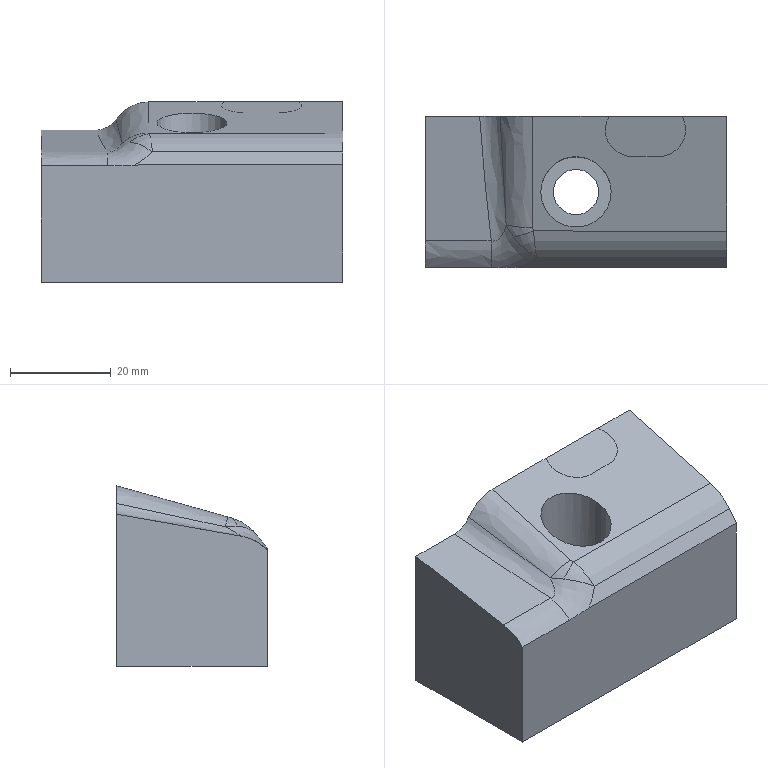Part | NX | features solid 2 | 1 solid | 19 faces | box 60 x 30 x 35.807 mm | volume 50490 mm3 | spline 10 | plane 7 | cylinder 2 | commonest cylinder face diameters 9 x1 14 x1
STEP:
#1=CARTESIAN_POINT('',(-520.5,-225.,15.));
#2=VERTEX_POINT('',#1);
#3=CARTESIAN_POINT('',(-525.,-225.,15.));
#4=DIRECTION('',(0.,0.,1.));
#5=DIRECTION('',(1.,0.,0.));
#6=AXIS2_PLACEMENT_3D('',#3,#4,#5);
#7=CIRCLE('',#6,4.5);
#8=EDGE_CURVE('',#2,#2,#7,.T.);
#9=ORIENTED_EDGE('',*,*,#8,.T.);
#10=EDGE_LOOP('',(#9));
#11=FACE_BOUND('',#10,.T.);
#12=CARTESIAN_POINT('',(-495.,-210.,15.));
#13=VERTEX_POINT('',#12);
#14=CARTESIAN_POINT('',(-555.,-210.,15.));
#15=VERTEX_POINT('',#14);
#16=CARTESIAN_POINT('',(-560.,-210.,15.));
#17=DIRECTION('',(-1.,0.,0.));
#18=VECTOR('',#17,1000.);
#19=LINE('',#16,#18);
#20=EDGE_CURVE('',#13,#15,#19,.T.);
#21=ORIENTED_EDGE('',*,*,#20,.F.);
#22=CARTESIAN_POINT('',(-495.,-240.,15.));
#23=VERTEX_POINT('',#22);
#24=CARTESIAN_POINT('',(-495.,-210.,15.));
#25=DIRECTION('',(0.,1.,0.));
#26=VECTOR('',#25,1000.);
#27=LINE('',#24,#26);
#28=EDGE_CURVE('',#23,#13,#27,.T.);
#29=ORIENTED_EDGE('',*,*,#28,.F.);
#30=CARTESIAN_POINT('',(-555.,-240.,15.));
#31=VERTEX_POINT('',#30);
#32=CARTESIAN_POINT('',(-485.,-240.,15.));
#33=DIRECTION('',(1.,0.,0.));
#34=VECTOR('',#33,1000.);
#35=LINE('',#32,#34);
#36=EDGE_CURVE('',#31,#23,#35,.T.);
#37=ORIENTED_EDGE('',*,*,#36,.F.);
#38=CARTESIAN_POINT('',(-555.,-240.,15.));
#39=DIRECTION('',(0.,-1.,0.));
#40=VECTOR('',#39,1000.);
#41=LINE('',#38,#40);
#42=EDGE_CURVE('',#15,#31,#41,.T.);
#43=ORIENTED_EDGE('',*,*,#42,.F.);
#44=EDGE_LOOP('',(#21,#29,#37,#43));
#45=FACE_BOUND('',#44,.T.);
#46=CARTESIAN_POINT('',(-525.,-45.,15.));
#47=DIRECTION('',(0.,0.,1.));
#48=DIRECTION('',(1.,0.,0.));
#49=AXIS2_PLACEMENT_3D('',#46,#47,#48);
#50=PLANE('',#49);
#51=ADVANCED_FACE('',(#11,#45),#50,.F.);
#52=CARTESIAN_POINT('',(-555.,-240.,38.085));
#53=VERTEX_POINT('',#52);
#54=CARTESIAN_POINT('',(-555.,-234.689,40.839));
#55=VERTEX_POINT('',#54);
#56=CARTESIAN_POINT('',(-555.,-240.,38.085));
#57=CARTESIAN_POINT('',(-555.,-238.554,39.522));
#58=CARTESIAN_POINT('',(-555.,-236.696,40.485));
#59=CARTESIAN_POINT('',(-555.,-234.689,40.839));
#60=B_SPLINE_CURVE_WITH_KNOTS('',3,(#56,#57,#58,#59),.UNSPECIFIED.,.F.,.F.,(4,4),(0.,0.006085),.UNSPECIFIED.);
#61=EDGE_CURVE('',#53,#55,#60,.T.);
#62=ORIENTED_EDGE('',*,*,#61,.T.);
#63=CARTESIAN_POINT('',(-555.,-210.,45.192));
#64=VERTEX_POINT('',#63);
#65=CARTESIAN_POINT('',(-555.,-255.374,37.192));
#66=DIRECTION('',(0.,-0.9848,-0.1736));
#67=VECTOR('',#66,1000.);
#68=LINE('',#65,#67);
#69=EDGE_CURVE('',#55,#64,#68,.F.);
#70=ORIENTED_EDGE('',*,*,#69,.T.);
#71=CARTESIAN_POINT('',(-555.,-210.,-50.));
#72=DIRECTION('',(0.,0.,1.));
#73=VECTOR('',#72,1000.);
#74=LINE('',#71,#73);
#75=EDGE_CURVE('',#15,#64,#74,.T.);
#76=ORIENTED_EDGE('',*,*,#75,.F.);
#77=ORIENTED_EDGE('',*,*,#42,.T.);
#78=CARTESIAN_POINT('',(-555.,-240.,-50.));
#79=DIRECTION('',(0.,0.,1.));
#80=VECTOR('',#79,1000.);
#81=LINE('',#78,#80);
#82=EDGE_CURVE('',#31,#53,#81,.T.);
#83=ORIENTED_EDGE('',*,*,#82,.T.);
#84=EDGE_LOOP('',(#62,#70,#76,#77,#83));
#85=FACE_BOUND('',#84,.T.);
#86=CARTESIAN_POINT('',(-555.,-240.,-50.));
#87=DIRECTION('',(1.,0.,0.));
#88=DIRECTION('',(0.,0.,-1.));
#89=AXIS2_PLACEMENT_3D('',#86,#87,#88);
#90=PLANE('',#89);
#91=ADVANCED_FACE('',(#85),#90,.F.);
#92=CARTESIAN_POINT('',(-536.45,-240.,38.268));
#93=VERTEX_POINT('',#92);
#94=CARTESIAN_POINT('',(-541.856,-240.,38.098));
#95=VERTEX_POINT('',#94);
#96=CARTESIAN_POINT('',(-536.45,-240.,38.268));
#97=CARTESIAN_POINT('',(-538.254,-240.,38.266));
#98=CARTESIAN_POINT('',(-540.052,-240.,38.1));
#99=CARTESIAN_POINT('',(-541.856,-240.,38.098));
#100=B_SPLINE_CURVE_WITH_KNOTS('',3,(#96,#97,#98,#99),.UNSPECIFIED.,.F.,.F.,(4,4),(0.,0.005409),.UNSPECIFIED.);
#101=EDGE_CURVE('',#93,#95,#100,.T.);
#102=ORIENTED_EDGE('',*,*,#101,.T.);
#103=CARTESIAN_POINT('',(-541.856,-240.,38.098));
#104=CARTESIAN_POINT('',(-546.237,-240.,38.094));
#105=CARTESIAN_POINT('',(-550.619,-240.,38.09));
#106=CARTESIAN_POINT('',(-555.,-240.,38.085));
#107=B_SPLINE_CURVE_WITH_KNOTS('',3,(#103,#104,#105,#106),.UNSPECIFIED.,.F.,.F.,(4,4),(0.,0.01314),.UNSPECIFIED.);
#108=EDGE_CURVE('',#95,#53,#107,.T.);
#109=ORIENTED_EDGE('',*,*,#108,.T.);
#110=ORIENTED_EDGE('',*,*,#82,.F.);
#111=ORIENTED_EDGE('',*,*,#36,.T.);
#112=CARTESIAN_POINT('',(-495.,-240.,38.323));
#113=VERTEX_POINT('',#112);
#114=CARTESIAN_POINT('',(-495.,-240.,-50.));
#115=DIRECTION('',(0.,0.,1.));
#116=VECTOR('',#115,1000.);
#117=LINE('',#114,#116);
#118=EDGE_CURVE('',#23,#113,#117,.T.);
#119=ORIENTED_EDGE('',*,*,#118,.T.);
#120=CARTESIAN_POINT('',(-485.117,-240.,38.336));
#121=DIRECTION('',(1.,0.,0.00132));
#122=VECTOR('',#121,1000.);
#123=LINE('',#120,#122);
#124=EDGE_CURVE('',#113,#93,#123,.F.);
#125=ORIENTED_EDGE('',*,*,#124,.T.);
#126=EDGE_LOOP('',(#102,#109,#110,#111,#119,#125));
#127=FACE_BOUND('',#126,.T.);
#128=CARTESIAN_POINT('',(-485.,-240.,-50.));
#129=DIRECTION('',(0.,1.,0.));
#130=DIRECTION('',(0.,0.,1.));
#131=AXIS2_PLACEMENT_3D('',#128,#129,#130);
#132=PLANE('',#131);
#133=ADVANCED_FACE('',(#127),#132,.F.);
#134=CARTESIAN_POINT('',(-495.,-232.81,44.429));
#135=VERTEX_POINT('',#134);
#136=CARTESIAN_POINT('',(-495.,-238.075,40.853));
#137=VERTEX_POINT('',#136);
#138=CARTESIAN_POINT('',(-495.,-232.81,44.429));
#139=CARTESIAN_POINT('',(-495.,-234.9,43.844));
#140=CARTESIAN_POINT('',(-495.,-236.761,42.581));
#141=CARTESIAN_POINT('',(-495.,-238.075,40.853));
#142=B_SPLINE_CURVE_WITH_KNOTS('',3,(#138,#139,#140,#141),.UNSPECIFIED.,.F.,.F.,(4,4),(0.,0.006489),.UNSPECIFIED.);
#143=EDGE_CURVE('',#135,#137,#142,.T.);
#144=ORIENTED_EDGE('',*,*,#143,.T.);
#145=CARTESIAN_POINT('',(-495.,-238.075,40.853));
#146=CARTESIAN_POINT('',(-495.,-238.717,40.01));
#147=CARTESIAN_POINT('',(-495.,-239.358,39.166));
#148=CARTESIAN_POINT('',(-495.,-240.,38.323));
#149=B_SPLINE_CURVE_WITH_KNOTS('',3,(#145,#146,#147,#148),.UNSPECIFIED.,.F.,.F.,(4,4),(0.000145,0.003324),.UNSPECIFIED.);
#150=EDGE_CURVE('',#137,#113,#149,.T.);
#151=ORIENTED_EDGE('',*,*,#150,.T.);
#152=ORIENTED_EDGE('',*,*,#118,.F.);
#153=ORIENTED_EDGE('',*,*,#28,.T.);
#154=CARTESIAN_POINT('',(-495.,-210.,50.807));
#155=VERTEX_POINT('',#154);
#156=CARTESIAN_POINT('',(-495.,-210.,-50.));
#157=DIRECTION('',(0.,0.,1.));
#158=VECTOR('',#157,1000.);
#159=LINE('',#156,#158);
#160=EDGE_CURVE('',#13,#155,#159,.T.);
#161=ORIENTED_EDGE('',*,*,#160,.T.);
#162=CARTESIAN_POINT('',(-495.,-236.145,43.496));
#163=DIRECTION('',(0.,-0.9631,-0.2693));
#164=VECTOR('',#163,1000.);
#165=LINE('',#162,#164);
#166=EDGE_CURVE('',#155,#135,#165,.T.);
#167=ORIENTED_EDGE('',*,*,#166,.T.);
#168=EDGE_LOOP('',(#144,#151,#152,#153,#161,#167));
#169=FACE_BOUND('',#168,.T.);
#170=CARTESIAN_POINT('',(-495.,-210.,-50.));
#171=DIRECTION('',(-1.,0.,0.));
#172=DIRECTION('',(0.,0.,1.));
#173=AXIS2_PLACEMENT_3D('',#170,#171,#172);
#174=PLANE('',#173);
#175=ADVANCED_FACE('',(#169),#174,.F.);
#176=ORIENTED_EDGE('',*,*,#75,.T.);
#177=CARTESIAN_POINT('',(-544.151,-210.,45.192));
#178=VERTEX_POINT('',#177);
#179=CARTESIAN_POINT('',(-560.,-210.,45.192));
#180=DIRECTION('',(-1.,0.,0.));
#181=VECTOR('',#180,1000.);
#182=LINE('',#179,#181);
#183=EDGE_CURVE('',#64,#178,#182,.F.);
#184=ORIENTED_EDGE('',*,*,#183,.T.);
#185=CARTESIAN_POINT('',(-540.089,-210.,47.332));
#186=VERTEX_POINT('',#185);
#187=CARTESIAN_POINT('',(-540.089,-210.,47.331));
#188=CARTESIAN_POINT('',(-541.,-210.,46.008));
#189=CARTESIAN_POINT('',(-542.544,-210.,45.192));
#190=CARTESIAN_POINT('',(-544.151,-210.,45.192));
#191=B_SPLINE_CURVE_WITH_KNOTS('',3,(#187,#188,#189,#190),.UNSPECIFIED.,.F.,.F.,(4,4),(0.,0.004781),.UNSPECIFIED.);
#192=EDGE_CURVE('',#186,#178,#191,.T.);
#193=ORIENTED_EDGE('',*,*,#192,.F.);
#194=CARTESIAN_POINT('',(-533.582,-210.,50.807));
#195=VERTEX_POINT('',#194);
#196=CARTESIAN_POINT('',(-540.089,-210.,47.332));
#197=CARTESIAN_POINT('',(-538.64,-210.,49.437));
#198=CARTESIAN_POINT('',(-536.169,-210.,50.807));
#199=CARTESIAN_POINT('',(-533.582,-210.,50.807));
#200=B_SPLINE_CURVE_WITH_KNOTS('',3,(#196,#197,#198,#199),.UNSPECIFIED.,.F.,.F.,(4,4),(0.0007923,0.008441),.UNSPECIFIED.);
#201=EDGE_CURVE('',#186,#195,#200,.T.);
#202=ORIENTED_EDGE('',*,*,#201,.T.);
#203=CARTESIAN_POINT('',(-518.42,-210.,50.807));
#204=VERTEX_POINT('',#203);
#205=CARTESIAN_POINT('',(-560.,-210.,50.807));
#206=DIRECTION('',(1.,0.,0.));
#207=VECTOR('',#206,1000.);
#208=LINE('',#205,#207);
#209=EDGE_CURVE('',#195,#204,#208,.T.);
#210=ORIENTED_EDGE('',*,*,#209,.T.);
#211=CARTESIAN_POINT('',(-503.958,-210.,50.807));
#212=VERTEX_POINT('',#211);
#213=CARTESIAN_POINT('',(-560.,-210.,50.807));
#214=DIRECTION('',(1.,0.,0.));
#215=VECTOR('',#214,1000.);
#216=LINE('',#213,#215);
#217=EDGE_CURVE('',#204,#212,#216,.T.);
#218=ORIENTED_EDGE('',*,*,#217,.T.);
#219=CARTESIAN_POINT('',(-560.,-210.,50.807));
#220=DIRECTION('',(1.,0.,0.));
#221=VECTOR('',#220,1000.);
#222=LINE('',#219,#221);
#223=EDGE_CURVE('',#212,#155,#222,.T.);
#224=ORIENTED_EDGE('',*,*,#223,.T.);
#225=ORIENTED_EDGE('',*,*,#160,.F.);
#226=ORIENTED_EDGE('',*,*,#20,.T.);
#227=EDGE_LOOP('',(#176,#184,#193,#202,#210,#218,#224,#225,#226));
#228=FACE_BOUND('',#227,.T.);
#229=CARTESIAN_POINT('',(-560.,-210.,-50.));
#230=DIRECTION('',(0.,-1.,0.));
#231=DIRECTION('',(0.,0.,-1.));
#232=AXIS2_PLACEMENT_3D('',#229,#230,#231);
#233=PLANE('',#232);
#234=ADVANCED_FACE('',(#228),#233,.F.);
#235=CARTESIAN_POINT('',(-538.881,-231.582,42.683));
#236=VERTEX_POINT('',#235);
#237=CARTESIAN_POINT('',(-538.881,-231.582,42.683));
#238=CARTESIAN_POINT('',(-539.385,-224.4,44.23));
#239=CARTESIAN_POINT('',(-539.769,-217.208,45.779));
#240=CARTESIAN_POINT('',(-540.089,-210.,47.331));
#241=B_SPLINE_CURVE_WITH_KNOTS('',3,(#237,#238,#239,#240),.UNSPECIFIED.,.F.,.F.,(4,4),(0.,0.7524),.UNSPECIFIED.);
#242=EDGE_CURVE('',#236,#186,#241,.T.);
#243=ORIENTED_EDGE('',*,*,#242,.T.);
#244=ORIENTED_EDGE('',*,*,#192,.T.);
#245=CARTESIAN_POINT('',(-541.849,-234.705,40.836));
#246=VERTEX_POINT('',#245);
#247=CARTESIAN_POINT('',(-544.151,-210.,45.192));
#248=CARTESIAN_POINT('',(-543.561,-218.253,43.737));
#249=CARTESIAN_POINT('',(-542.843,-226.478,42.287));
#250=CARTESIAN_POINT('',(-541.849,-234.705,40.836));
#251=B_SPLINE_CURVE_WITH_KNOTS('',3,(#247,#248,#249,#250),.UNSPECIFIED.,.F.,.F.,(4,4),(0.2271,1.),.UNSPECIFIED.);
#252=EDGE_CURVE('',#246,#178,#251,.F.);
#253=ORIENTED_EDGE('',*,*,#252,.F.);
#254=CARTESIAN_POINT('',(-541.849,-234.705,40.836));
#255=CARTESIAN_POINT('',(-540.548,-235.001,40.784));
#256=CARTESIAN_POINT('',(-539.539,-233.948,41.415));
#257=CARTESIAN_POINT('',(-538.881,-231.582,42.683));
#258=B_SPLINE_CURVE_WITH_KNOTS('',3,(#254,#255,#256,#257),.UNSPECIFIED.,.F.,.F.,(4,4),(0.,1.),.UNSPECIFIED.);
#259=EDGE_CURVE('',#246,#236,#258,.T.);
#260=ORIENTED_EDGE('',*,*,#259,.T.);
#261=EDGE_LOOP('',(#243,#244,#253,#260));
#262=FACE_BOUND('',#261,.T.);
#263=CARTESIAN_POINT('',(-538.631,-235.011,41.944));
#264=CARTESIAN_POINT('',(-539.159,-234.998,41.5));
#265=CARTESIAN_POINT('',(-539.763,-235.009,41.145));
#266=CARTESIAN_POINT('',(-540.421,-235.046,40.897));
#267=CARTESIAN_POINT('',(-541.106,-235.106,40.766));
#268=CARTESIAN_POINT('',(-541.791,-235.187,40.751));
#269=CARTESIAN_POINT('',(-538.635,-234.953,41.956));
#270=CARTESIAN_POINT('',(-539.164,-234.939,41.512));
#271=CARTESIAN_POINT('',(-539.768,-234.95,41.157));
#272=CARTESIAN_POINT('',(-540.426,-234.986,40.908));
#273=CARTESIAN_POINT('',(-541.112,-235.047,40.776));
#274=CARTESIAN_POINT('',(-541.798,-235.128,40.762));
#275=CARTESIAN_POINT('',(-538.64,-234.894,41.969));
#276=CARTESIAN_POINT('',(-539.168,-234.88,41.524));
#277=CARTESIAN_POINT('',(-539.773,-234.891,41.168));
#278=CARTESIAN_POINT('',(-540.432,-234.927,40.918));
#279=CARTESIAN_POINT('',(-541.119,-234.988,40.786));
#280=CARTESIAN_POINT('',(-541.805,-235.069,40.772));
#281=CARTESIAN_POINT('',(-538.644,-234.835,41.982));
#282=CARTESIAN_POINT('',(-539.173,-234.821,41.536));
#283=CARTESIAN_POINT('',(-539.778,-234.832,41.179));
#284=CARTESIAN_POINT('',(-540.438,-234.868,40.929));
#285=CARTESIAN_POINT('',(-541.125,-234.928,40.797));
#286=CARTESIAN_POINT('',(-541.812,-235.01,40.783));
#287=CARTESIAN_POINT('',(-538.648,-234.777,41.994));
#288=CARTESIAN_POINT('',(-539.178,-234.762,41.548));
#289=CARTESIAN_POINT('',(-539.783,-234.773,41.19));
#290=CARTESIAN_POINT('',(-540.444,-234.809,40.94));
#291=CARTESIAN_POINT('',(-541.132,-234.869,40.807));
#292=CARTESIAN_POINT('',(-541.82,-234.95,40.793));
#293=CARTESIAN_POINT('',(-538.653,-234.718,42.007));
#294=CARTESIAN_POINT('',(-539.182,-234.703,41.559));
#295=CARTESIAN_POINT('',(-539.788,-234.714,41.201));
#296=CARTESIAN_POINT('',(-540.449,-234.75,40.951));
#297=CARTESIAN_POINT('',(-541.138,-234.81,40.818));
#298=CARTESIAN_POINT('',(-541.827,-234.891,40.804));
#299=CARTESIAN_POINT('',(-538.949,-230.798,42.851));
#300=CARTESIAN_POINT('',(-539.495,-230.769,42.35));
#301=CARTESIAN_POINT('',(-540.131,-230.768,41.947));
#302=CARTESIAN_POINT('',(-540.835,-230.796,41.664));
#303=CARTESIAN_POINT('',(-541.571,-230.851,41.516));
#304=CARTESIAN_POINT('',(-542.308,-230.93,41.502));
#305=CARTESIAN_POINT('',(-539.209,-226.879,43.695));
#306=CARTESIAN_POINT('',(-539.765,-226.837,43.141));
#307=CARTESIAN_POINT('',(-540.427,-226.825,42.693));
#308=CARTESIAN_POINT('',(-541.168,-226.844,42.378));
#309=CARTESIAN_POINT('',(-541.949,-226.894,42.214));
#310=CARTESIAN_POINT('',(-542.73,-226.97,42.2));
#311=CARTESIAN_POINT('',(-539.443,-222.973,44.537));
#312=CARTESIAN_POINT('',(-540.003,-222.918,43.931));
#313=CARTESIAN_POINT('',(-540.687,-222.894,43.437));
#314=CARTESIAN_POINT('',(-541.464,-222.905,43.09));
#315=CARTESIAN_POINT('',(-542.286,-222.95,42.909));
#316=CARTESIAN_POINT('',(-543.109,-223.024,42.896));
#317=CARTESIAN_POINT('',(-539.713,-217.991,45.61));
#318=CARTESIAN_POINT('',(-540.274,-217.919,44.939));
#319=CARTESIAN_POINT('',(-540.981,-217.881,44.387));
#320=CARTESIAN_POINT('',(-541.799,-217.881,43.998));
#321=CARTESIAN_POINT('',(-542.673,-217.919,43.796));
#322=CARTESIAN_POINT('',(-543.547,-217.99,43.784));
#323=CARTESIAN_POINT('',(-539.952,-213.005,46.684));
#324=CARTESIAN_POINT('',(-540.508,-212.918,45.949));
#325=CARTESIAN_POINT('',(-541.233,-212.865,45.339));
#326=CARTESIAN_POINT('',(-542.09,-212.854,44.906));
#327=CARTESIAN_POINT('',(-543.012,-212.885,44.684));
#328=CARTESIAN_POINT('',(-543.935,-212.953,44.672));
#329=CARTESIAN_POINT('',(-540.002,-211.954,46.91));
#330=CARTESIAN_POINT('',(-540.555,-211.863,46.162));
#331=CARTESIAN_POINT('',(-541.285,-211.807,45.54));
#332=CARTESIAN_POINT('',(-542.149,-211.794,45.098));
#333=CARTESIAN_POINT('',(-543.082,-211.823,44.871));
#334=CARTESIAN_POINT('',(-544.015,-211.89,44.859));
#335=CARTESIAN_POINT('',(-540.049,-210.902,47.137));
#336=CARTESIAN_POINT('',(-540.602,-210.808,46.376));
#337=CARTESIAN_POINT('',(-541.334,-210.749,45.741));
#338=CARTESIAN_POINT('',(-542.207,-210.733,45.29));
#339=CARTESIAN_POINT('',(-543.149,-210.761,45.058));
#340=CARTESIAN_POINT('',(-544.092,-210.827,45.047));
#341=CARTESIAN_POINT('',(-540.096,-209.85,47.363));
#342=CARTESIAN_POINT('',(-540.646,-209.753,46.589));
#343=CARTESIAN_POINT('',(-541.382,-209.691,45.942));
#344=CARTESIAN_POINT('',(-542.262,-209.673,45.482));
#345=CARTESIAN_POINT('',(-543.215,-209.699,45.246));
#346=CARTESIAN_POINT('',(-544.168,-209.765,45.234));
#347=B_SPLINE_SURFACE_WITH_KNOTS('',5,5,((#263,#264,#265,#266,#267,#268),(#269,#270,#271,#272,#273,#274),(#275,#276,#277,#278,#279,#280),(#281,#282,#283,#284,#285,#286),(#287,#288,#289,#290,#291,#292),(#293,#294,#295,#296,#297,#298),(#299,#300,#301,#302,#303,#304),(#305,#306,#307,#308,#309,#310),(#311,#312,#313,#314,#315,#316),(#317,#318,#319,#320,#321,#322),(#323,#324,#325,#326,#327,#328),(#329,#330,#331,#332,#333,#334),(#335,#336,#337,#338,#339,#340),(#341,#342,#343,#344,#345,#346)),.UNSPECIFIED.,.F.,.F.,.F.,(6,5,3,6),(6,6),(0.0007587,0.009901,0.6205,0.7837),(0.,1.),.UNSPECIFIED.);
#348=ADVANCED_FACE('',(#262),#347,.T.);
#349=ORIENTED_EDGE('',*,*,#201,.F.);
#350=ORIENTED_EDGE('',*,*,#242,.F.);
#351=CARTESIAN_POINT('',(-533.576,-232.122,44.621));
#352=VERTEX_POINT('',#351);
#353=CARTESIAN_POINT('',(-538.881,-231.582,42.683));
#354=CARTESIAN_POINT('',(-537.423,-231.929,43.927));
#355=CARTESIAN_POINT('',(-535.412,-232.123,44.621));
#356=CARTESIAN_POINT('',(-533.576,-232.122,44.621));
#357=B_SPLINE_CURVE_WITH_KNOTS('',3,(#353,#354,#355,#356),.UNSPECIFIED.,.F.,.F.,(4,4),(0.,1.),.UNSPECIFIED.);
#358=EDGE_CURVE('',#236,#352,#357,.T.);
#359=ORIENTED_EDGE('',*,*,#358,.T.);
#360=CARTESIAN_POINT('',(-533.576,-232.122,44.621));
#361=CARTESIAN_POINT('',(-533.578,-224.748,46.683));
#362=CARTESIAN_POINT('',(-533.58,-217.374,48.745));
#363=CARTESIAN_POINT('',(-533.582,-210.,50.807));
#364=B_SPLINE_CURVE_WITH_KNOTS('',3,(#360,#361,#362,#363),.UNSPECIFIED.,.F.,.F.,(4,4),(0.,0.3805),.UNSPECIFIED.);
#365=EDGE_CURVE('',#352,#195,#364,.T.);
#366=ORIENTED_EDGE('',*,*,#365,.T.);
#367=EDGE_LOOP('',(#349,#350,#359,#366));
#368=FACE_BOUND('',#367,.T.);
#369=CARTESIAN_POINT('',(-540.109,-231.213,41.362));
#370=CARTESIAN_POINT('',(-540.115,-208.958,47.586));
#371=CARTESIAN_POINT('',(-538.573,-231.798,43.455));
#372=CARTESIAN_POINT('',(-538.579,-209.542,49.679));
#373=CARTESIAN_POINT('',(-536.215,-232.123,44.621));
#374=CARTESIAN_POINT('',(-536.221,-209.868,50.844));
#375=CARTESIAN_POINT('',(-533.576,-232.122,44.621));
#376=CARTESIAN_POINT('',(-533.582,-209.867,50.844));
#377=(BOUNDED_SURFACE()B_SPLINE_SURFACE(3,1,((#369,#370),(#371,#372),(#373,#374),(#375,#376)),.CYLINDRICAL_SURF.,.F.,.F.,.F.)B_SPLINE_SURFACE_WITH_KNOTS((4,4),(2,2),(0.09053,1.),(0.,0.2437),.PIECEWISE_BEZIER_KNOTS.)GEOMETRIC_REPRESENTATION_ITEM()RATIONAL_B_SPLINE_SURFACE(((0.9779,0.9779),(0.9114,0.9114),(0.9188,0.9188),(1.,1.)))REPRESENTATION_ITEM('')SURFACE());
#378=ADVANCED_FACE('',(#368),#377,.T.);
#379=ORIENTED_EDGE('',*,*,#217,.F.);
#380=CARTESIAN_POINT('',(-513.689,-218.,48.57));
#381=VERTEX_POINT('',#380);
#382=CARTESIAN_POINT('',(-518.42,-210.,50.807));
#383=CARTESIAN_POINT('',(-518.909,-210.796,50.585));
#384=CARTESIAN_POINT('',(-519.45,-212.653,50.065));
#385=CARTESIAN_POINT('',(-518.443,-216.398,49.018));
#386=CARTESIAN_POINT('',(-515.645,-218.,48.57));
#387=CARTESIAN_POINT('',(-513.689,-218.,48.57));
#388=B_SPLINE_CURVE_WITH_KNOTS('',3,(#382,#383,#384,#385,#386,#387),.UNSPECIFIED.,.F.,.F.,(4,1,1,4),(0.3296,0.4972,0.6648,1.),.UNSPECIFIED.);
#389=EDGE_CURVE('',#204,#381,#388,.T.);
#390=ORIENTED_EDGE('',*,*,#389,.T.);
#391=CARTESIAN_POINT('',(-508.689,-218.,48.57));
#392=VERTEX_POINT('',#391);
#393=CARTESIAN_POINT('',(-513.689,-218.,48.57));
#394=CARTESIAN_POINT('',(-512.022,-218.,48.57));
#395=CARTESIAN_POINT('',(-510.356,-218.,48.57));
#396=CARTESIAN_POINT('',(-508.689,-218.,48.57));
#397=B_SPLINE_CURVE_WITH_KNOTS('',3,(#393,#394,#395,#396),.UNSPECIFIED.,.F.,.F.,(4,4),(0.,1.),.UNSPECIFIED.);
#398=EDGE_CURVE('',#381,#392,#397,.T.);
#399=ORIENTED_EDGE('',*,*,#398,.T.);
#400=CARTESIAN_POINT('',(-508.689,-218.,48.57));
#401=CARTESIAN_POINT('',(-506.732,-218.,48.57));
#402=CARTESIAN_POINT('',(-503.935,-216.397,49.018));
#403=CARTESIAN_POINT('',(-502.928,-212.653,50.065));
#404=CARTESIAN_POINT('',(-503.469,-210.796,50.585));
#405=CARTESIAN_POINT('',(-503.958,-210.,50.807));
#406=B_SPLINE_CURVE_WITH_KNOTS('',3,(#400,#401,#402,#403,#404,#405),.UNSPECIFIED.,.F.,.F.,(4,1,1,4),(0.,0.3352,0.5028,0.6704),.UNSPECIFIED.);
#407=EDGE_CURVE('',#392,#212,#406,.T.);
#408=ORIENTED_EDGE('',*,*,#407,.T.);
#409=EDGE_LOOP('',(#379,#390,#399,#408));
#410=FACE_BOUND('',#409,.T.);
#411=CARTESIAN_POINT('',(-519.285,-218.,48.57));
#412=CARTESIAN_POINT('',(-503.093,-218.,48.57));
#413=CARTESIAN_POINT('',(-519.285,-210.,50.807));
#414=CARTESIAN_POINT('',(-503.093,-210.,50.807));
#415=B_SPLINE_SURFACE_WITH_KNOTS('',1,1,((#411,#412),(#413,#414)),.PLANE_SURF.,.F.,.F.,.F.,(2,2),(2,2),(0.1496,0.2265),(0.116,0.2405),.PIECEWISE_BEZIER_KNOTS.);
#416=ADVANCED_FACE('',(#410),#415,.F.);
#417=ORIENTED_EDGE('',*,*,#143,.F.);
#418=CARTESIAN_POINT('',(-533.461,-232.761,44.442));
#419=VERTEX_POINT('',#418);
#420=CARTESIAN_POINT('',(-495.,-232.81,44.429));
#421=CARTESIAN_POINT('',(-507.82,-232.793,44.433));
#422=CARTESIAN_POINT('',(-520.641,-232.777,44.438));
#423=CARTESIAN_POINT('',(-533.461,-232.761,44.442));
#424=B_SPLINE_CURVE_WITH_KNOTS('',3,(#420,#421,#422,#423),.UNSPECIFIED.,.F.,.F.,(4,4),(0.2476,1.),.UNSPECIFIED.);
#425=EDGE_CURVE('',#135,#419,#424,.T.);
#426=ORIENTED_EDGE('',*,*,#425,.T.);
#427=CARTESIAN_POINT('',(-532.863,-238.027,40.867));
#428=VERTEX_POINT('',#427);
#429=CARTESIAN_POINT('',(-533.461,-232.761,44.442));
#430=CARTESIAN_POINT('',(-533.262,-234.804,43.871));
#431=CARTESIAN_POINT('',(-533.063,-236.742,42.555));
#432=CARTESIAN_POINT('',(-532.863,-238.027,40.867));
#433=B_SPLINE_CURVE_WITH_KNOTS('',3,(#429,#430,#431,#432),.UNSPECIFIED.,.F.,.F.,(4,4),(0.,1.),.UNSPECIFIED.);
#434=EDGE_CURVE('',#419,#428,#433,.T.);
#435=ORIENTED_EDGE('',*,*,#434,.T.);
#436=CARTESIAN_POINT('',(-532.863,-238.027,40.867));
#437=CARTESIAN_POINT('',(-520.242,-238.043,40.862));
#438=CARTESIAN_POINT('',(-507.621,-238.059,40.858));
#439=CARTESIAN_POINT('',(-495.,-238.075,40.853));
#440=B_SPLINE_CURVE_WITH_KNOTS('',3,(#436,#437,#438,#439),.UNSPECIFIED.,.F.,.F.,(4,4),(0.,0.7496),.UNSPECIFIED.);
#441=EDGE_CURVE('',#137,#428,#440,.F.);
#442=ORIENTED_EDGE('',*,*,#441,.F.);
#443=EDGE_LOOP('',(#417,#426,#435,#442));
#444=FACE_BOUND('',#443,.T.);
#445=CARTESIAN_POINT('',(-533.692,-232.76,44.442));
#446=CARTESIAN_POINT('',(-494.761,-232.81,44.429));
#447=CARTESIAN_POINT('',(-533.695,-234.877,43.851));
#448=CARTESIAN_POINT('',(-494.764,-234.927,43.837));
#449=CARTESIAN_POINT('',(-533.698,-236.695,42.616));
#450=CARTESIAN_POINT('',(-494.767,-236.745,42.602));
#451=CARTESIAN_POINT('',(-533.7,-238.026,40.867));
#452=CARTESIAN_POINT('',(-494.769,-238.075,40.853));
#453=(BOUNDED_SURFACE()B_SPLINE_SURFACE(3,1,((#445,#446),(#447,#448),(#449,#450),(#451,#452)),.CYLINDRICAL_SURF.,.F.,.F.,.F.)B_SPLINE_SURFACE_WITH_KNOTS((4,4),(2,2),(0.,1.),(0.001476,0.7585),.PIECEWISE_BEZIER_KNOTS.)GEOMETRIC_REPRESENTATION_ITEM()RATIONAL_B_SPLINE_SURFACE(((1.,1.),(0.9653,0.9653),(0.9653,0.9653),(1.,1.)))REPRESENTATION_ITEM('')SURFACE());
#454=ADVANCED_FACE('',(#444),#453,.T.);
#455=CARTESIAN_POINT('',(-525.,-218.,48.57));
#456=VERTEX_POINT('',#455);
#457=CARTESIAN_POINT('',(-525.,-225.,46.613));
#458=DIRECTION('',(0.,0.2693,-0.9631));
#459=DIRECTION('',(0.,0.9631,0.2693));
#460=AXIS2_PLACEMENT_3D('',#457,#458,#459);
#461=ELLIPSE('',#460,7.269,7.);
#462=EDGE_CURVE('',#456,#456,#461,.T.);
#463=ORIENTED_EDGE('',*,*,#462,.T.);
#464=EDGE_LOOP('',(#463));
#465=FACE_BOUND('',#464,.T.);
#466=ORIENTED_EDGE('',*,*,#209,.F.);
#467=ORIENTED_EDGE('',*,*,#365,.F.);
#468=CARTESIAN_POINT('',(-533.461,-232.761,44.442));
#469=CARTESIAN_POINT('',(-533.537,-232.581,44.493));
#470=CARTESIAN_POINT('',(-533.575,-232.368,44.552));
#471=CARTESIAN_POINT('',(-533.576,-232.122,44.621));
#472=B_SPLINE_CURVE_WITH_KNOTS('',3,(#468,#469,#470,#471),.UNSPECIFIED.,.F.,.F.,(4,4),(0.,1.),.UNSPECIFIED.);
#473=EDGE_CURVE('',#352,#419,#472,.F.);
#474=ORIENTED_EDGE('',*,*,#473,.T.);
#475=ORIENTED_EDGE('',*,*,#425,.F.);
#476=ORIENTED_EDGE('',*,*,#166,.F.);
#477=ORIENTED_EDGE('',*,*,#223,.F.);
#478=ORIENTED_EDGE('',*,*,#407,.F.);
#479=ORIENTED_EDGE('',*,*,#398,.F.);
#480=ORIENTED_EDGE('',*,*,#389,.F.);
#481=EDGE_LOOP('',(#466,#467,#474,#475,#476,#477,#478,#479,#480));
#482=FACE_BOUND('',#481,.T.);
#483=CARTESIAN_POINT('',(-571.189,-212.817,50.02));
#484=DIRECTION('',(0.,0.2693,-0.9631));
#485=DIRECTION('',(0.,0.9631,0.2693));
#486=AXIS2_PLACEMENT_3D('',#483,#484,#485);
#487=PLANE('',#486);
#488=ADVANCED_FACE('',(#465,#482),#487,.F.);
#489=ORIENTED_EDGE('',*,*,#150,.F.);
#490=ORIENTED_EDGE('',*,*,#441,.T.);
#491=CARTESIAN_POINT('',(-532.863,-238.027,40.867));
#492=CARTESIAN_POINT('',(-533.928,-238.857,39.774));
#493=CARTESIAN_POINT('',(-535.124,-239.514,38.908));
#494=CARTESIAN_POINT('',(-536.45,-240.,38.268));
#495=B_SPLINE_CURVE_WITH_KNOTS('',3,(#491,#492,#493,#494),.UNSPECIFIED.,.F.,.F.,(4,4),(0.,0.4816),.UNSPECIFIED.);
#496=EDGE_CURVE('',#428,#93,#495,.T.);
#497=ORIENTED_EDGE('',*,*,#496,.T.);
#498=ORIENTED_EDGE('',*,*,#124,.F.);
#499=EDGE_LOOP('',(#489,#490,#497,#498));
#500=FACE_BOUND('',#499,.T.);
#501=CARTESIAN_POINT('',(-536.699,-238.012,40.88));
#502=CARTESIAN_POINT('',(-495.,-238.039,40.901));
#503=CARTESIAN_POINT('',(-536.699,-240.012,38.253));
#504=CARTESIAN_POINT('',(-495.,-240.038,38.273));
#505=B_SPLINE_SURFACE_WITH_KNOTS('',1,1,((#501,#502),(#503,#504)),.PLANE_SURF.,.F.,.F.,.F.,(2,2),(2,2),(0.004824,0.1912),(0.3826,0.8518),.PIECEWISE_BEZIER_KNOTS.);
#506=ADVANCED_FACE('',(#500),#505,.T.);
#507=ORIENTED_EDGE('',*,*,#101,.F.);
#508=ORIENTED_EDGE('',*,*,#496,.F.);
#509=CARTESIAN_POINT('',(-537.39,-233.979,42.836));
#510=VERTEX_POINT('',#509);
#511=CARTESIAN_POINT('',(-537.39,-233.979,42.836));
#512=CARTESIAN_POINT('',(-536.04,-235.723,42.741));
#513=CARTESIAN_POINT('',(-534.404,-237.14,42.031));
#514=CARTESIAN_POINT('',(-532.863,-238.027,40.867));
#515=B_SPLINE_CURVE_WITH_KNOTS('',3,(#511,#512,#513,#514),.UNSPECIFIED.,.F.,.F.,(4,4),(0.,1.),.UNSPECIFIED.);
#516=EDGE_CURVE('',#510,#428,#515,.T.);
#517=ORIENTED_EDGE('',*,*,#516,.F.);
#518=CARTESIAN_POINT('',(-538.881,-231.582,42.683));
#519=CARTESIAN_POINT('',(-538.466,-232.434,42.826));
#520=CARTESIAN_POINT('',(-537.965,-233.24,42.874));
#521=CARTESIAN_POINT('',(-537.39,-233.979,42.836));
#522=B_SPLINE_CURVE_WITH_KNOTS('',3,(#518,#519,#520,#521),.UNSPECIFIED.,.F.,.F.,(4,4),(0.,1.),.UNSPECIFIED.);
#523=EDGE_CURVE('',#236,#510,#522,.T.);
#524=ORIENTED_EDGE('',*,*,#523,.F.);
#525=ORIENTED_EDGE('',*,*,#259,.F.);
#526=CARTESIAN_POINT('',(-541.856,-240.,38.098));
#527=CARTESIAN_POINT('',(-541.854,-238.565,39.517));
#528=CARTESIAN_POINT('',(-541.852,-236.692,40.486));
#529=CARTESIAN_POINT('',(-541.849,-234.705,40.836));
#530=B_SPLINE_CURVE_WITH_KNOTS('',3,(#526,#527,#528,#529),.UNSPECIFIED.,.F.,.F.,(4,4),(0.1884,1.),.UNSPECIFIED.);
#531=EDGE_CURVE('',#95,#246,#530,.T.);
#532=ORIENTED_EDGE('',*,*,#531,.F.);
#533=EDGE_LOOP('',(#507,#508,#517,#524,#525,#532));
#534=FACE_BOUND('',#533,.T.);
#535=CARTESIAN_POINT('',(-541.849,-234.705,40.836));
#536=CARTESIAN_POINT('',(-541.851,-236.174,40.577));
#537=CARTESIAN_POINT('',(-541.853,-237.595,40.044));
#538=CARTESIAN_POINT('',(-541.854,-238.899,39.249));
#539=CARTESIAN_POINT('',(-541.856,-240.023,38.23));
#540=CARTESIAN_POINT('',(-541.857,-240.927,37.043));
#541=CARTESIAN_POINT('',(-541.53,-234.778,40.823));
#542=CARTESIAN_POINT('',(-541.432,-236.23,40.556));
#543=CARTESIAN_POINT('',(-541.318,-237.634,40.021));
#544=CARTESIAN_POINT('',(-541.191,-238.922,39.229));
#545=CARTESIAN_POINT('',(-541.058,-240.033,38.219));
#546=CARTESIAN_POINT('',(-540.924,-240.928,37.043));
#547=CARTESIAN_POINT('',(-541.211,-234.781,40.847));
#548=CARTESIAN_POINT('',(-541.012,-236.221,40.586));
#549=CARTESIAN_POINT('',(-540.778,-237.611,40.06));
#550=CARTESIAN_POINT('',(-540.52,-238.885,39.281));
#551=CARTESIAN_POINT('',(-540.249,-239.983,38.286));
#552=CARTESIAN_POINT('',(-539.979,-240.865,37.126));
#553=CARTESIAN_POINT('',(-540.905,-234.703,40.912));
#554=CARTESIAN_POINT('',(-540.603,-236.137,40.674));
#555=CARTESIAN_POINT('',(-540.251,-237.517,40.172));
#556=CARTESIAN_POINT('',(-539.863,-238.78,39.416));
#557=CARTESIAN_POINT('',(-539.455,-239.864,38.443));
#558=CARTESIAN_POINT('',(-539.047,-240.731,37.304));
#559=CARTESIAN_POINT('',(-540.16,-234.308,41.176));
#560=CARTESIAN_POINT('',(-539.61,-235.738,41.036));
#561=CARTESIAN_POINT('',(-538.962,-237.108,40.627));
#562=CARTESIAN_POINT('',(-538.243,-238.351,39.955));
#563=CARTESIAN_POINT('',(-537.487,-239.401,39.054));
#564=CARTESIAN_POINT('',(-536.732,-240.221,37.978));
#565=CARTESIAN_POINT('',(-539.586,-233.503,41.639));
#566=CARTESIAN_POINT('',(-538.848,-234.963,41.672));
#567=CARTESIAN_POINT('',(-537.956,-236.356,41.419));
#568=CARTESIAN_POINT('',(-536.949,-237.598,40.879));
#569=CARTESIAN_POINT('',(-535.885,-238.62,40.083));
#570=CARTESIAN_POINT('',(-534.82,-239.379,39.087));
#571=CARTESIAN_POINT('',(-539.305,-232.911,41.966));
#572=CARTESIAN_POINT('',(-538.484,-234.401,42.119));
#573=CARTESIAN_POINT('',(-537.468,-235.817,41.976));
#574=CARTESIAN_POINT('',(-536.307,-237.067,41.527));
#575=CARTESIAN_POINT('',(-535.072,-238.074,40.802));
#576=CARTESIAN_POINT('',(-533.837,-238.793,39.859));
#577=CARTESIAN_POINT('',(-539.071,-232.266,42.316));
#578=CARTESIAN_POINT('',(-538.191,-233.792,42.595));
#579=CARTESIAN_POINT('',(-537.071,-235.236,42.569));
#580=CARTESIAN_POINT('',(-535.77,-236.499,42.218));
#581=CARTESIAN_POINT('',(-534.378,-237.492,41.568));
#582=CARTESIAN_POINT('',(-532.986,-238.17,40.679));
#583=CARTESIAN_POINT('',(-538.881,-231.582,42.683));
#584=CARTESIAN_POINT('',(-537.963,-233.149,43.088));
#585=CARTESIAN_POINT('',(-536.759,-234.629,43.182));
#586=CARTESIAN_POINT('',(-535.333,-235.908,42.934));
#587=CARTESIAN_POINT('',(-533.795,-236.887,42.363));
#588=CARTESIAN_POINT('',(-532.257,-237.523,41.53));
#589=B_SPLINE_SURFACE_WITH_KNOTS('',5,5,((#535,#536,#537,#538,#539,#540),(#541,#542,#543,#544,#545,#546),(#547,#548,#549,#550,#551,#552),(#553,#554,#555,#556,#557,#558),(#559,#560,#561,#562,#563,#564),(#565,#566,#567,#568,#569,#570),(#571,#572,#573,#574,#575,#576),(#577,#578,#579,#580,#581,#582),(#583,#584,#585,#586,#587,#588)),.UNSPECIFIED.,.F.,.F.,.F.,(6,3,6),(6,6),(0.,0.3808,1.),(0.,1.),.UNSPECIFIED.);
#590=ADVANCED_FACE('',(#534),#589,.F.);
#591=ORIENTED_EDGE('',*,*,#183,.F.);
#592=ORIENTED_EDGE('',*,*,#69,.F.);
#593=CARTESIAN_POINT('',(-545.41,-234.701,40.837));
#594=VERTEX_POINT('',#593);
#595=CARTESIAN_POINT('',(-555.,-234.689,40.839));
#596=CARTESIAN_POINT('',(-551.803,-234.693,40.838));
#597=CARTESIAN_POINT('',(-548.607,-234.697,40.838));
#598=CARTESIAN_POINT('',(-545.41,-234.701,40.837));
#599=B_SPLINE_CURVE_WITH_KNOTS('',3,(#595,#596,#597,#598),.UNSPECIFIED.,.F.,.F.,(4,4),(0.6126,1.),.UNSPECIFIED.);
#600=EDGE_CURVE('',#55,#594,#599,.T.);
#601=ORIENTED_EDGE('',*,*,#600,.T.);
#602=CARTESIAN_POINT('',(-545.41,-234.701,40.837));
#603=CARTESIAN_POINT('',(-544.223,-234.702,40.837));
#604=CARTESIAN_POINT('',(-543.036,-234.703,40.837));
#605=CARTESIAN_POINT('',(-541.849,-234.705,40.836));
#606=B_SPLINE_CURVE_WITH_KNOTS('',3,(#602,#603,#604,#605),.UNSPECIFIED.,.F.,.F.,(4,4),(0.,1.),.UNSPECIFIED.);
#607=EDGE_CURVE('',#594,#246,#606,.T.);
#608=ORIENTED_EDGE('',*,*,#607,.T.);
#609=ORIENTED_EDGE('',*,*,#252,.T.);
#610=EDGE_LOOP('',(#591,#592,#601,#608,#609));
#611=FACE_BOUND('',#610,.T.);
#612=CARTESIAN_POINT('',(-555.,-210.,45.192));
#613=CARTESIAN_POINT('',(-541.77,-210.,45.192));
#614=CARTESIAN_POINT('',(-555.,-234.853,40.81));
#615=CARTESIAN_POINT('',(-541.77,-234.853,40.81));
#616=B_SPLINE_SURFACE_WITH_KNOTS('',1,1,((#612,#613),(#614,#615)),.PLANE_SURF.,.F.,.F.,.F.,(2,2),(2,2),(0.07329,0.3239),(0.9091,0.9945),.PIECEWISE_BEZIER_KNOTS.);
#617=ADVANCED_FACE('',(#611),#616,.T.);
#618=ORIENTED_EDGE('',*,*,#108,.F.);
#619=ORIENTED_EDGE('',*,*,#531,.T.);
#620=ORIENTED_EDGE('',*,*,#607,.F.);
#621=ORIENTED_EDGE('',*,*,#600,.F.);
#622=ORIENTED_EDGE('',*,*,#61,.F.);
#623=EDGE_LOOP('',(#618,#619,#620,#621,#622));
#624=FACE_BOUND('',#623,.T.);
#625=CARTESIAN_POINT('',(-555.079,-234.689,40.839));
#626=CARTESIAN_POINT('',(-541.849,-234.705,40.836));
#627=CARTESIAN_POINT('',(-555.081,-236.72,40.481));
#628=CARTESIAN_POINT('',(-541.852,-236.735,40.478));
#629=CARTESIAN_POINT('',(-555.084,-238.558,39.529));
#630=CARTESIAN_POINT('',(-541.854,-238.573,39.526));
#631=CARTESIAN_POINT('',(-555.086,-240.026,38.06));
#632=CARTESIAN_POINT('',(-541.856,-240.041,38.057));
#633=(BOUNDED_SURFACE()B_SPLINE_SURFACE(3,1,((#625,#626),(#627,#628),(#629,#630),(#631,#632)),.CYLINDRICAL_SURF.,.F.,.F.,.F.)B_SPLINE_SURFACE_WITH_KNOTS((4,4),(2,2),(0.,0.8172),(0.5328,1.),.PIECEWISE_BEZIER_KNOTS.)GEOMETRIC_REPRESENTATION_ITEM()RATIONAL_B_SPLINE_SURFACE(((1.,1.),(0.9626,0.9626),(0.9557,0.9557),(0.9795,0.9795)))REPRESENTATION_ITEM('')SURFACE());
#634=ADVANCED_FACE('',(#624),#633,.T.);
#635=ORIENTED_EDGE('',*,*,#523,.T.);
#636=CARTESIAN_POINT('',(-537.39,-233.979,42.836));
#637=CARTESIAN_POINT('',(-536.22,-233.731,43.727));
#638=CARTESIAN_POINT('',(-534.842,-233.304,44.29));
#639=CARTESIAN_POINT('',(-533.461,-232.761,44.442));
#640=B_SPLINE_CURVE_WITH_KNOTS('',3,(#636,#637,#638,#639),.UNSPECIFIED.,.F.,.F.,(4,4),(0.,1.),.UNSPECIFIED.);
#641=EDGE_CURVE('',#419,#510,#640,.F.);
#642=ORIENTED_EDGE('',*,*,#641,.F.);
#643=ORIENTED_EDGE('',*,*,#473,.F.);
#644=ORIENTED_EDGE('',*,*,#358,.F.);
#645=EDGE_LOOP('',(#635,#642,#643,#644));
#646=FACE_BOUND('',#645,.T.);
#647=CARTESIAN_POINT('',(-537.39,-233.979,42.836));
#648=CARTESIAN_POINT('',(-536.688,-233.83,43.371));
#649=CARTESIAN_POINT('',(-535.924,-233.629,43.81));
#650=CARTESIAN_POINT('',(-535.118,-233.379,44.14));
#651=CARTESIAN_POINT('',(-534.289,-233.087,44.351));
#652=CARTESIAN_POINT('',(-533.461,-232.761,44.442));
#653=CARTESIAN_POINT('',(-537.734,-233.536,42.859));
#654=CARTESIAN_POINT('',(-536.986,-233.456,43.413));
#655=CARTESIAN_POINT('',(-536.166,-233.323,43.863));
#656=CARTESIAN_POINT('',(-535.297,-233.141,44.195));
#657=CARTESIAN_POINT('',(-534.402,-232.915,44.399));
#658=CARTESIAN_POINT('',(-533.507,-232.653,44.473));
#659=CARTESIAN_POINT('',(-538.057,-233.073,42.856));
#660=CARTESIAN_POINT('',(-537.268,-233.063,43.44));
#661=CARTESIAN_POINT('',(-536.395,-233.002,43.911));
#662=CARTESIAN_POINT('',(-535.464,-232.89,44.252));
#663=CARTESIAN_POINT('',(-534.503,-232.732,44.45));
#664=CARTESIAN_POINT('',(-533.541,-232.534,44.506));
#665=CARTESIAN_POINT('',(-538.357,-232.59,42.826));
#666=CARTESIAN_POINT('',(-537.534,-232.653,43.452));
#667=CARTESIAN_POINT('',(-536.611,-232.666,43.952));
#668=CARTESIAN_POINT('',(-535.619,-232.627,44.308));
#669=CARTESIAN_POINT('',(-534.592,-232.539,44.504));
#670=CARTESIAN_POINT('',(-533.564,-232.406,44.542));
#671=CARTESIAN_POINT('',(-538.633,-232.092,42.768));
#672=CARTESIAN_POINT('',(-537.782,-232.227,43.446));
#673=CARTESIAN_POINT('',(-536.815,-232.316,43.987));
#674=CARTESIAN_POINT('',(-535.763,-232.352,44.363));
#675=CARTESIAN_POINT('',(-534.669,-232.335,44.561));
#676=CARTESIAN_POINT('',(-533.576,-232.268,44.58));
#677=CARTESIAN_POINT('',(-538.881,-231.582,42.683));
#678=CARTESIAN_POINT('',(-538.013,-231.789,43.424));
#679=CARTESIAN_POINT('',(-537.005,-231.953,44.013));
#680=CARTESIAN_POINT('',(-535.896,-232.066,44.418));
#681=CARTESIAN_POINT('',(-534.736,-232.122,44.621));
#682=CARTESIAN_POINT('',(-533.576,-232.122,44.621));
#683=B_SPLINE_SURFACE_WITH_KNOTS('',5,5,((#647,#648,#649,#650,#651,#652),(#653,#654,#655,#656,#657,#658),(#659,#660,#661,#662,#663,#664),(#665,#666,#667,#668,#669,#670),(#671,#672,#673,#674,#675,#676),(#677,#678,#679,#680,#681,#682)),.UNSPECIFIED.,.F.,.F.,.F.,(6,6),(6,6),(0.,1.),(0.,1.),.PIECEWISE_BEZIER_KNOTS.);
#684=ADVANCED_FACE('',(#646),#683,.F.);
#685=ORIENTED_EDGE('',*,*,#641,.T.);
#686=ORIENTED_EDGE('',*,*,#516,.T.);
#687=ORIENTED_EDGE('',*,*,#434,.F.);
#688=EDGE_LOOP('',(#685,#686,#687));
#689=FACE_BOUND('',#688,.T.);
#690=CARTESIAN_POINT('',(-537.39,-233.979,42.836));
#691=CARTESIAN_POINT('',(-536.688,-233.83,43.371));
#692=CARTESIAN_POINT('',(-535.924,-233.629,43.81));
#693=CARTESIAN_POINT('',(-535.118,-233.379,44.14));
#694=CARTESIAN_POINT('',(-534.289,-233.087,44.351));
#695=CARTESIAN_POINT('',(-533.461,-232.761,44.442));
#696=CARTESIAN_POINT('',(-536.047,-235.706,42.753));
#697=CARTESIAN_POINT('',(-535.498,-235.618,43.042));
#698=CARTESIAN_POINT('',(-534.946,-235.49,43.297));
#699=CARTESIAN_POINT('',(-534.393,-235.322,43.518));
#700=CARTESIAN_POINT('',(-533.839,-235.114,43.706));
#701=CARTESIAN_POINT('',(-533.285,-234.868,43.858));
#702=CARTESIAN_POINT('',(-534.419,-237.136,42.044));
#703=CARTESIAN_POINT('',(-534.148,-237.054,42.144));
#704=CARTESIAN_POINT('',(-533.878,-236.973,42.246));
#705=CARTESIAN_POINT('',(-533.608,-236.893,42.351));
#706=CARTESIAN_POINT('',(-533.339,-236.815,42.458));
#707=CARTESIAN_POINT('',(-533.07,-236.738,42.568));
#708=CARTESIAN_POINT('',(-532.863,-238.027,40.867));
#709=CARTESIAN_POINT('',(-532.863,-238.027,40.867));
#710=CARTESIAN_POINT('',(-532.863,-238.027,40.867));
#711=CARTESIAN_POINT('',(-532.863,-238.027,40.867));
#712=CARTESIAN_POINT('',(-532.863,-238.027,40.867));
#713=CARTESIAN_POINT('',(-532.863,-238.027,40.867));
#714=B_SPLINE_SURFACE_WITH_KNOTS('',3,5,((#690,#691,#692,#693,#694,#695),(#696,#697,#698,#699,#700,#701),(#702,#703,#704,#705,#706,#707),(#708,#709,#710,#711,#712,#713)),.UNSPECIFIED.,.F.,.F.,.F.,(4,4),(6,6),(0.,1.),(0.,1.),.PIECEWISE_BEZIER_KNOTS.);
#715=ADVANCED_FACE('',(#689),#714,.T.);
#716=CARTESIAN_POINT('',(-529.5,-225.,25.));
#717=VERTEX_POINT('',#716);
#718=CARTESIAN_POINT('',(-525.,-225.,25.));
#719=DIRECTION('',(0.,0.,-1.));
#720=DIRECTION('',(-1.,0.,0.));
#721=AXIS2_PLACEMENT_3D('',#718,#719,#720);
#722=CIRCLE('',#721,4.5);
#723=EDGE_CURVE('',#717,#717,#722,.T.);
#724=ORIENTED_EDGE('',*,*,#723,.F.);
#725=EDGE_LOOP('',(#724));
#726=FACE_BOUND('',#725,.T.);
#727=ORIENTED_EDGE('',*,*,#8,.F.);
#728=EDGE_LOOP('',(#727));
#729=FACE_BOUND('',#728,.T.);
#730=CARTESIAN_POINT('',(-525.,-225.,25.));
#731=DIRECTION('',(0.,0.,-1.));
#732=DIRECTION('',(-1.,0.,0.));
#733=AXIS2_PLACEMENT_3D('',#730,#731,#732);
#734=CYLINDRICAL_SURFACE('',#733,4.5);
#735=ADVANCED_FACE('',(#726,#729),#734,.F.);
#736=CARTESIAN_POINT('',(-518.,-225.,25.));
#737=VERTEX_POINT('',#736);
#738=CARTESIAN_POINT('',(-525.,-225.,25.));
#739=DIRECTION('',(0.,0.,1.));
#740=DIRECTION('',(1.,0.,0.));
#741=AXIS2_PLACEMENT_3D('',#738,#739,#740);
#742=CIRCLE('',#741,7.);
#743=EDGE_CURVE('',#737,#737,#742,.T.);
#744=ORIENTED_EDGE('',*,*,#743,.F.);
#745=EDGE_LOOP('',(#744));
#746=FACE_BOUND('',#745,.T.);
#747=ORIENTED_EDGE('',*,*,#462,.F.);
#748=EDGE_LOOP('',(#747));
#749=FACE_BOUND('',#748,.T.);
#750=CARTESIAN_POINT('',(-525.,-225.,25.));
#751=DIRECTION('',(0.,0.,1.));
#752=DIRECTION('',(1.,0.,0.));
#753=AXIS2_PLACEMENT_3D('',#750,#751,#752);
#754=CYLINDRICAL_SURFACE('',#753,7.);
#755=ADVANCED_FACE('',(#746,#749),#754,.F.);
#756=ORIENTED_EDGE('',*,*,#723,.T.);
#757=EDGE_LOOP('',(#756));
#758=FACE_BOUND('',#757,.T.);
#759=ORIENTED_EDGE('',*,*,#743,.T.);
#760=EDGE_LOOP('',(#759));
#761=FACE_BOUND('',#760,.T.);
#762=CARTESIAN_POINT('',(-525.,-225.,25.));
#763=DIRECTION('',(0.,0.,-1.));
#764=DIRECTION('',(-1.,0.,0.));
#765=AXIS2_PLACEMENT_3D('',#762,#763,#764);
#766=PLANE('',#765);
#767=ADVANCED_FACE('',(#758,#761),#766,.F.);
#768=CLOSED_SHELL('',(#51,#91,#133,#175,#234,#348,#378,#416,#454,#488,#506,#590,#617,#634,#684,#715,#735,#755,#767));
#769=MANIFOLD_SOLID_BREP('',#768);
#770=(LENGTH_UNIT()NAMED_UNIT(*)SI_UNIT(.MILLI.,.METRE.));
#771=UNCERTAINTY_MEASURE_WITH_UNIT(LENGTH_MEASURE(0.05184),#770,'','');
#772=(NAMED_UNIT(*)PLANE_ANGLE_UNIT()SI_UNIT($,.RADIAN.));
#773=(NAMED_UNIT(*)SI_UNIT($,.STERADIAN.)SOLID_ANGLE_UNIT());
#774=(GEOMETRIC_REPRESENTATION_CONTEXT(3)GLOBAL_UNCERTAINTY_ASSIGNED_CONTEXT((#771))GLOBAL_UNIT_ASSIGNED_CONTEXT((#770,#772,#773))REPRESENTATION_CONTEXT('',''));
#775=ADVANCED_BREP_SHAPE_REPRESENTATION('',(#769),#774);